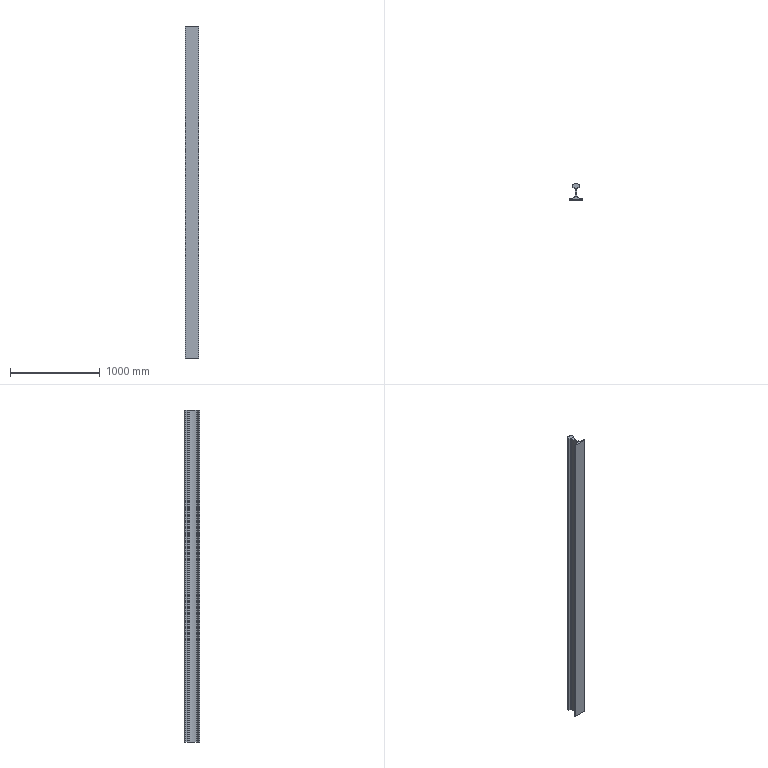Part | STEP file | 60 rail | 1 solid | 33 faces | box 150 x 176.167 x 3700 mm | volume 28206021 mm3 | cylinder 18 | plane 13 | spline 2 | commonest cylinder face diameters 4 x5 16 x2 26 x2 40 x2 50 x2 80 x2
STEP:
#1=CARTESIAN_POINT('',(-102.213,32.964,3700.));
#2=VERTEX_POINT('',#1);
#3=CARTESIAN_POINT('',(-103.574,34.86,3700.));
#4=VERTEX_POINT('',#3);
#5=CARTESIAN_POINT('',(-101.574,34.86,3700.));
#6=DIRECTION('',(0.,0.,-1.));
#7=DIRECTION('',(1.,0.,0.));
#8=AXIS2_PLACEMENT_3D('',#5,#6,#7);
#9=CIRCLE('',#8,2.);
#10=EDGE_CURVE('',#2,#4,#9,.T.);
#11=ORIENTED_EDGE('',*,*,#10,.T.);
#12=CARTESIAN_POINT('',(-103.574,34.86,0.));
#13=VERTEX_POINT('',#12);
#14=CARTESIAN_POINT('',(-103.574,34.86,3700.));
#15=DIRECTION('',(0.,0.,-1.));
#16=VECTOR('',#15,1000.);
#17=LINE('',#14,#16);
#18=EDGE_CURVE('',#4,#13,#17,.T.);
#19=ORIENTED_EDGE('',*,*,#18,.T.);
#20=CARTESIAN_POINT('',(-102.213,32.964,0.));
#21=VERTEX_POINT('',#20);
#22=CARTESIAN_POINT('',(-101.574,34.86,0.));
#23=DIRECTION('',(0.,0.,-1.));
#24=DIRECTION('',(1.,0.,0.));
#25=AXIS2_PLACEMENT_3D('',#22,#23,#24);
#26=CIRCLE('',#25,2.);
#27=EDGE_CURVE('',#21,#13,#26,.T.);
#28=ORIENTED_EDGE('',*,*,#27,.F.);
#29=CARTESIAN_POINT('',(-102.213,32.964,3700.));
#30=DIRECTION('',(0.,0.,-1.));
#31=VECTOR('',#30,1000.);
#32=LINE('',#29,#31);
#33=EDGE_CURVE('',#2,#21,#32,.T.);
#34=ORIENTED_EDGE('',*,*,#33,.F.);
#35=EDGE_LOOP('',(#11,#19,#28,#34));
#36=FACE_OUTER_BOUND('',#35,.T.);
#37=CARTESIAN_POINT('',(-101.574,34.86,3700.));
#38=DIRECTION('',(0.,0.,-1.));
#39=DIRECTION('',(-1.,0.,0.));
#40=AXIS2_PLACEMENT_3D('',#37,#38,#39);
#41=CYLINDRICAL_SURFACE('',#40,2.);
#42=ADVANCED_FACE('',(#36),#41,.T.);
#43=CARTESIAN_POINT('',(-80.306,23.184,0.));
#44=VERTEX_POINT('',#43);
#45=CARTESIAN_POINT('',(-77.547,14.047,0.));
#46=VERTEX_POINT('',#45);
#47=CARTESIAN_POINT('',(-102.419,11.522,0.));
#48=DIRECTION('',(0.,0.,-1.));
#49=DIRECTION('',(1.,0.,0.));
#50=AXIS2_PLACEMENT_3D('',#47,#48,#49);
#51=CIRCLE('',#50,25.);
#52=EDGE_CURVE('',#44,#46,#51,.T.);
#53=ORIENTED_EDGE('',*,*,#52,.T.);
#54=CARTESIAN_POINT('',(-77.547,14.047,3700.));
#55=VERTEX_POINT('',#54);
#56=CARTESIAN_POINT('',(-77.547,14.047,3700.));
#57=DIRECTION('',(0.,0.,-1.));
#58=VECTOR('',#57,1000.);
#59=LINE('',#56,#58);
#60=EDGE_CURVE('',#55,#46,#59,.T.);
#61=ORIENTED_EDGE('',*,*,#60,.F.);
#62=CARTESIAN_POINT('',(-80.306,23.184,3700.));
#63=VERTEX_POINT('',#62);
#64=CARTESIAN_POINT('',(-102.419,11.522,3700.));
#65=DIRECTION('',(0.,0.,-1.));
#66=DIRECTION('',(1.,0.,0.));
#67=AXIS2_PLACEMENT_3D('',#64,#65,#66);
#68=CIRCLE('',#67,25.);
#69=EDGE_CURVE('',#63,#55,#68,.T.);
#70=ORIENTED_EDGE('',*,*,#69,.F.);
#71=CARTESIAN_POINT('',(-80.306,23.184,3700.));
#72=DIRECTION('',(0.,0.,-1.));
#73=VECTOR('',#72,1000.);
#74=LINE('',#71,#73);
#75=EDGE_CURVE('',#63,#44,#74,.T.);
#76=ORIENTED_EDGE('',*,*,#75,.T.);
#77=EDGE_LOOP('',(#53,#61,#70,#76));
#78=FACE_OUTER_BOUND('',#77,.T.);
#79=CARTESIAN_POINT('',(-102.419,11.522,3700.));
#80=DIRECTION('',(0.,0.,-1.));
#81=DIRECTION('',(-1.,0.,0.));
#82=AXIS2_PLACEMENT_3D('',#79,#80,#81);
#83=CYLINDRICAL_SURFACE('',#82,25.);
#84=ADVANCED_FACE('',(#78),#83,.F.);
#85=CARTESIAN_POINT('',(-77.347,-66.653,0.));
#86=VERTEX_POINT('',#85);
#87=CARTESIAN_POINT('',(-77.547,14.047,0.));
#88=CARTESIAN_POINT('',(-70.798,-27.011,0.));
#89=CARTESIAN_POINT('',(-77.347,-66.653,0.));
#90=B_SPLINE_CURVE_WITH_KNOTS('',2,(#87,#88,#89),.UNSPECIFIED.,.F.,.F.,(3,3),(0.,0.7644),.UNSPECIFIED.);
#91=EDGE_CURVE('',#46,#86,#90,.T.);
#92=ORIENTED_EDGE('',*,*,#91,.T.);
#93=CARTESIAN_POINT('',(-77.347,-66.653,3700.));
#94=VERTEX_POINT('',#93);
#95=CARTESIAN_POINT('',(-77.347,-66.653,3700.));
#96=DIRECTION('',(0.,0.,-1.));
#97=VECTOR('',#96,1000.);
#98=LINE('',#95,#97);
#99=EDGE_CURVE('',#94,#86,#98,.T.);
#100=ORIENTED_EDGE('',*,*,#99,.F.);
#101=CARTESIAN_POINT('',(-77.547,14.047,3700.));
#102=CARTESIAN_POINT('',(-70.798,-27.011,3700.));
#103=CARTESIAN_POINT('',(-77.347,-66.653,3700.));
#104=B_SPLINE_CURVE_WITH_KNOTS('',2,(#101,#102,#103),.UNSPECIFIED.,.F.,.F.,(3,3),(0.,0.7644),.UNSPECIFIED.);
#105=EDGE_CURVE('',#55,#94,#104,.T.);
#106=ORIENTED_EDGE('',*,*,#105,.F.);
#107=ORIENTED_EDGE('',*,*,#60,.T.);
#108=EDGE_LOOP('',(#92,#100,#106,#107));
#109=FACE_OUTER_BOUND('',#108,.T.);
#110=CARTESIAN_POINT('',(-77.547,14.047,3700.));
#111=CARTESIAN_POINT('',(-77.547,14.047,0.));
#112=CARTESIAN_POINT('',(-70.798,-27.011,3700.));
#113=CARTESIAN_POINT('',(-70.798,-27.011,0.));
#114=CARTESIAN_POINT('',(-77.347,-66.653,3700.));
#115=CARTESIAN_POINT('',(-77.347,-66.653,0.));
#116=B_SPLINE_SURFACE_WITH_KNOTS('',2,1,((#110,#111),(#112,#113),(#114,#115)),.UNSPECIFIED.,.F.,.F.,.F.,(3,3),(2,2),(0.,0.7644),(0.,1.),.UNSPECIFIED.);
#117=ADVANCED_FACE('',(#109),#116,.F.);
#118=CARTESIAN_POINT('',(-90.947,-83.653,0.));
#119=VERTEX_POINT('',#118);
#120=CARTESIAN_POINT('',(-97.249,-64.671,0.));
#121=DIRECTION('',(0.,0.,-1.));
#122=DIRECTION('',(1.,0.,0.));
#123=AXIS2_PLACEMENT_3D('',#120,#121,#122);
#124=CIRCLE('',#123,20.);
#125=EDGE_CURVE('',#86,#119,#124,.T.);
#126=ORIENTED_EDGE('',*,*,#125,.T.);
#127=CARTESIAN_POINT('',(-90.947,-83.653,3700.));
#128=VERTEX_POINT('',#127);
#129=CARTESIAN_POINT('',(-90.947,-83.653,3700.));
#130=DIRECTION('',(0.,0.,-1.));
#131=VECTOR('',#130,1000.);
#132=LINE('',#129,#131);
#133=EDGE_CURVE('',#128,#119,#132,.T.);
#134=ORIENTED_EDGE('',*,*,#133,.F.);
#135=CARTESIAN_POINT('',(-97.249,-64.671,3700.));
#136=DIRECTION('',(0.,0.,-1.));
#137=DIRECTION('',(1.,0.,0.));
#138=AXIS2_PLACEMENT_3D('',#135,#136,#137);
#139=CIRCLE('',#138,20.);
#140=EDGE_CURVE('',#94,#128,#139,.T.);
#141=ORIENTED_EDGE('',*,*,#140,.F.);
#142=ORIENTED_EDGE('',*,*,#99,.T.);
#143=EDGE_LOOP('',(#126,#134,#141,#142));
#144=FACE_OUTER_BOUND('',#143,.T.);
#145=CARTESIAN_POINT('',(-97.249,-64.671,3700.));
#146=DIRECTION('',(0.,0.,-1.));
#147=DIRECTION('',(-1.,0.,0.));
#148=AXIS2_PLACEMENT_3D('',#145,#146,#147);
#149=CYLINDRICAL_SURFACE('',#148,20.);
#150=ADVANCED_FACE('',(#144),#149,.F.);
#151=CARTESIAN_POINT('',(-108.856,-89.622,0.));
#152=VERTEX_POINT('',#151);
#153=CARTESIAN_POINT('',(16.001,-48.003,0.));
#154=DIRECTION('',(-0.9487,-0.3162,0.));
#155=VECTOR('',#154,1000.);
#156=LINE('',#153,#155);
#157=EDGE_CURVE('',#119,#152,#156,.T.);
#158=ORIENTED_EDGE('',*,*,#157,.T.);
#159=CARTESIAN_POINT('',(-108.856,-89.622,3700.));
#160=VERTEX_POINT('',#159);
#161=CARTESIAN_POINT('',(-108.856,-89.622,3700.));
#162=DIRECTION('',(0.,0.,-1.));
#163=VECTOR('',#162,1000.);
#164=LINE('',#161,#163);
#165=EDGE_CURVE('',#160,#152,#164,.T.);
#166=ORIENTED_EDGE('',*,*,#165,.F.);
#167=CARTESIAN_POINT('',(16.001,-48.003,3700.));
#168=DIRECTION('',(-0.9487,-0.3162,0.));
#169=VECTOR('',#168,1000.);
#170=LINE('',#167,#169);
#171=EDGE_CURVE('',#128,#160,#170,.T.);
#172=ORIENTED_EDGE('',*,*,#171,.F.);
#173=ORIENTED_EDGE('',*,*,#133,.T.);
#174=EDGE_LOOP('',(#158,#166,#172,#173));
#175=FACE_OUTER_BOUND('',#174,.T.);
#176=CARTESIAN_POINT('',(16.001,-48.003,3700.));
#177=DIRECTION('',(0.3162,-0.9487,0.));
#178=DIRECTION('',(0.9487,0.3162,0.));
#179=AXIS2_PLACEMENT_3D('',#176,#177,#178);
#180=PLANE('',#179);
#181=ADVANCED_FACE('',(#175),#180,.F.);
#182=CARTESIAN_POINT('',(-117.028,-91.423,0.));
#183=VERTEX_POINT('',#182);
#184=CARTESIAN_POINT('',(-121.505,-51.675,0.));
#185=DIRECTION('',(0.,0.,1.));
#186=DIRECTION('',(1.,0.,0.));
#187=AXIS2_PLACEMENT_3D('',#184,#185,#186);
#188=CIRCLE('',#187,40.);
#189=EDGE_CURVE('',#183,#152,#188,.T.);
#190=ORIENTED_EDGE('',*,*,#189,.F.);
#191=CARTESIAN_POINT('',(-117.028,-91.423,3700.));
#192=VERTEX_POINT('',#191);
#193=CARTESIAN_POINT('',(-117.028,-91.423,3700.));
#194=DIRECTION('',(0.,0.,-1.));
#195=VECTOR('',#194,1000.);
#196=LINE('',#193,#195);
#197=EDGE_CURVE('',#192,#183,#196,.T.);
#198=ORIENTED_EDGE('',*,*,#197,.F.);
#199=CARTESIAN_POINT('',(-121.505,-51.675,3700.));
#200=DIRECTION('',(0.,0.,1.));
#201=DIRECTION('',(1.,0.,0.));
#202=AXIS2_PLACEMENT_3D('',#199,#200,#201);
#203=CIRCLE('',#202,40.);
#204=EDGE_CURVE('',#192,#160,#203,.T.);
#205=ORIENTED_EDGE('',*,*,#204,.T.);
#206=ORIENTED_EDGE('',*,*,#165,.T.);
#207=EDGE_LOOP('',(#190,#198,#205,#206));
#208=FACE_OUTER_BOUND('',#207,.T.);
#209=CARTESIAN_POINT('',(-121.505,-51.675,3700.));
#210=DIRECTION('',(0.,0.,-1.));
#211=DIRECTION('',(-1.,0.,0.));
#212=AXIS2_PLACEMENT_3D('',#209,#210,#211);
#213=CYLINDRICAL_SURFACE('',#212,40.);
#214=ADVANCED_FACE('',(#208),#213,.F.);
#215=CARTESIAN_POINT('',(-140.371,-94.052,0.));
#216=VERTEX_POINT('',#215);
#217=CARTESIAN_POINT('',(8.702,-77.263,0.));
#218=DIRECTION('',(-0.9937,-0.1119,0.));
#219=VECTOR('',#218,1000.);
#220=LINE('',#217,#219);
#221=EDGE_CURVE('',#183,#216,#220,.T.);
#222=ORIENTED_EDGE('',*,*,#221,.T.);
#223=CARTESIAN_POINT('',(-140.371,-94.052,3700.));
#224=VERTEX_POINT('',#223);
#225=CARTESIAN_POINT('',(-140.371,-94.052,3700.));
#226=DIRECTION('',(0.,0.,-1.));
#227=VECTOR('',#226,1000.);
#228=LINE('',#225,#227);
#229=EDGE_CURVE('',#224,#216,#228,.T.);
#230=ORIENTED_EDGE('',*,*,#229,.F.);
#231=CARTESIAN_POINT('',(8.702,-77.263,3700.));
#232=DIRECTION('',(-0.9937,-0.1119,0.));
#233=VECTOR('',#232,1000.);
#234=LINE('',#231,#233);
#235=EDGE_CURVE('',#192,#224,#234,.T.);
#236=ORIENTED_EDGE('',*,*,#235,.F.);
#237=ORIENTED_EDGE('',*,*,#197,.T.);
#238=EDGE_LOOP('',(#222,#230,#236,#237));
#239=FACE_OUTER_BOUND('',#238,.T.);
#240=CARTESIAN_POINT('',(8.702,-77.263,3700.));
#241=DIRECTION('',(0.1119,-0.9937,0.));
#242=DIRECTION('',(0.9937,0.1119,0.));
#243=AXIS2_PLACEMENT_3D('',#240,#241,#242);
#244=PLANE('',#243);
#245=ADVANCED_FACE('',(#239),#244,.F.);
#246=CARTESIAN_POINT('',(-142.147,-96.04,0.));
#247=VERTEX_POINT('',#246);
#248=CARTESIAN_POINT('',(-140.147,-96.04,0.));
#249=DIRECTION('',(0.,0.,-1.));
#250=DIRECTION('',(1.,0.,0.));
#251=AXIS2_PLACEMENT_3D('',#248,#249,#250);
#252=CIRCLE('',#251,2.);
#253=EDGE_CURVE('',#247,#216,#252,.T.);
#254=ORIENTED_EDGE('',*,*,#253,.F.);
#255=CARTESIAN_POINT('',(-142.147,-96.04,3700.));
#256=VERTEX_POINT('',#255);
#257=CARTESIAN_POINT('',(-142.147,-96.04,3700.));
#258=DIRECTION('',(0.,0.,-1.));
#259=VECTOR('',#258,1000.);
#260=LINE('',#257,#259);
#261=EDGE_CURVE('',#256,#247,#260,.T.);
#262=ORIENTED_EDGE('',*,*,#261,.F.);
#263=CARTESIAN_POINT('',(-140.147,-96.04,3700.));
#264=DIRECTION('',(0.,0.,-1.));
#265=DIRECTION('',(1.,0.,0.));
#266=AXIS2_PLACEMENT_3D('',#263,#264,#265);
#267=CIRCLE('',#266,2.);
#268=EDGE_CURVE('',#256,#224,#267,.T.);
#269=ORIENTED_EDGE('',*,*,#268,.T.);
#270=ORIENTED_EDGE('',*,*,#229,.T.);
#271=EDGE_LOOP('',(#254,#262,#269,#270));
#272=FACE_OUTER_BOUND('',#271,.T.);
#273=CARTESIAN_POINT('',(-140.147,-96.04,3700.));
#274=DIRECTION('',(0.,0.,-1.));
#275=DIRECTION('',(-1.,0.,0.));
#276=AXIS2_PLACEMENT_3D('',#273,#274,#275);
#277=CYLINDRICAL_SURFACE('',#276,2.);
#278=ADVANCED_FACE('',(#272),#277,.T.);
#279=CARTESIAN_POINT('',(-142.147,-106.253,0.));
#280=VERTEX_POINT('',#279);
#281=CARTESIAN_POINT('',(-142.147,0.,0.));
#282=DIRECTION('',(0.,1.,0.));
#283=VECTOR('',#282,1000.);
#284=LINE('',#281,#283);
#285=EDGE_CURVE('',#280,#247,#284,.T.);
#286=ORIENTED_EDGE('',*,*,#285,.F.);
#287=CARTESIAN_POINT('',(-142.147,-106.253,3700.));
#288=VERTEX_POINT('',#287);
#289=CARTESIAN_POINT('',(-142.147,-106.253,3700.));
#290=DIRECTION('',(0.,0.,-1.));
#291=VECTOR('',#290,1000.);
#292=LINE('',#289,#291);
#293=EDGE_CURVE('',#288,#280,#292,.T.);
#294=ORIENTED_EDGE('',*,*,#293,.F.);
#295=CARTESIAN_POINT('',(-142.147,0.,3700.));
#296=DIRECTION('',(0.,1.,0.));
#297=VECTOR('',#296,1000.);
#298=LINE('',#295,#297);
#299=EDGE_CURVE('',#288,#256,#298,.T.);
#300=ORIENTED_EDGE('',*,*,#299,.T.);
#301=ORIENTED_EDGE('',*,*,#261,.T.);
#302=EDGE_LOOP('',(#286,#294,#300,#301));
#303=FACE_OUTER_BOUND('',#302,.T.);
#304=CARTESIAN_POINT('',(-142.147,0.,3700.));
#305=DIRECTION('',(-1.,0.,0.));
#306=DIRECTION('',(0.,0.,1.));
#307=AXIS2_PLACEMENT_3D('',#304,#305,#306);
#308=PLANE('',#307);
#309=ADVANCED_FACE('',(#303),#308,.T.);
#310=CARTESIAN_POINT('',(7.853,-106.253,0.));
#311=VERTEX_POINT('',#310);
#312=CARTESIAN_POINT('',(0.,-106.253,0.));
#313=DIRECTION('',(1.,0.,0.));
#314=VECTOR('',#313,1000.);
#315=LINE('',#312,#314);
#316=EDGE_CURVE('',#280,#311,#315,.T.);
#317=ORIENTED_EDGE('',*,*,#316,.T.);
#318=CARTESIAN_POINT('',(7.853,-106.253,3700.));
#319=VERTEX_POINT('',#318);
#320=CARTESIAN_POINT('',(7.853,-106.253,3700.));
#321=DIRECTION('',(0.,0.,-1.));
#322=VECTOR('',#321,1000.);
#323=LINE('',#320,#322);
#324=EDGE_CURVE('',#319,#311,#323,.T.);
#325=ORIENTED_EDGE('',*,*,#324,.F.);
#326=CARTESIAN_POINT('',(0.,-106.253,3700.));
#327=DIRECTION('',(1.,0.,0.));
#328=VECTOR('',#327,1000.);
#329=LINE('',#326,#328);
#330=EDGE_CURVE('',#288,#319,#329,.T.);
#331=ORIENTED_EDGE('',*,*,#330,.F.);
#332=ORIENTED_EDGE('',*,*,#293,.T.);
#333=EDGE_LOOP('',(#317,#325,#331,#332));
#334=FACE_OUTER_BOUND('',#333,.T.);
#335=CARTESIAN_POINT('',(0.,-106.253,3700.));
#336=DIRECTION('',(0.,1.,0.));
#337=DIRECTION('',(0.,0.,1.));
#338=AXIS2_PLACEMENT_3D('',#335,#336,#337);
#339=PLANE('',#338);
#340=ADVANCED_FACE('',(#334),#339,.F.);
#341=CARTESIAN_POINT('',(7.853,-96.04,0.));
#342=VERTEX_POINT('',#341);
#343=CARTESIAN_POINT('',(7.853,0.,0.));
#344=DIRECTION('',(0.,1.,0.));
#345=VECTOR('',#344,1000.);
#346=LINE('',#343,#345);
#347=EDGE_CURVE('',#311,#342,#346,.T.);
#348=ORIENTED_EDGE('',*,*,#347,.T.);
#349=CARTESIAN_POINT('',(7.853,-96.04,3700.));
#350=VERTEX_POINT('',#349);
#351=CARTESIAN_POINT('',(7.853,-96.04,3700.));
#352=DIRECTION('',(0.,0.,-1.));
#353=VECTOR('',#352,1000.);
#354=LINE('',#351,#353);
#355=EDGE_CURVE('',#350,#342,#354,.T.);
#356=ORIENTED_EDGE('',*,*,#355,.F.);
#357=CARTESIAN_POINT('',(7.853,0.,3700.));
#358=DIRECTION('',(0.,1.,0.));
#359=VECTOR('',#358,1000.);
#360=LINE('',#357,#359);
#361=EDGE_CURVE('',#319,#350,#360,.T.);
#362=ORIENTED_EDGE('',*,*,#361,.F.);
#363=ORIENTED_EDGE('',*,*,#324,.T.);
#364=EDGE_LOOP('',(#348,#356,#362,#363));
#365=FACE_OUTER_BOUND('',#364,.T.);
#366=CARTESIAN_POINT('',(7.853,0.,3700.));
#367=DIRECTION('',(-1.,0.,0.));
#368=DIRECTION('',(0.,0.,1.));
#369=AXIS2_PLACEMENT_3D('',#366,#367,#368);
#370=PLANE('',#369);
#371=ADVANCED_FACE('',(#365),#370,.F.);
#372=CARTESIAN_POINT('',(6.077,-94.052,0.));
#373=VERTEX_POINT('',#372);
#374=CARTESIAN_POINT('',(5.853,-96.04,0.));
#375=DIRECTION('',(0.,0.,1.));
#376=DIRECTION('',(1.,0.,0.));
#377=AXIS2_PLACEMENT_3D('',#374,#375,#376);
#378=CIRCLE('',#377,2.);
#379=EDGE_CURVE('',#342,#373,#378,.T.);
#380=ORIENTED_EDGE('',*,*,#379,.T.);
#381=CARTESIAN_POINT('',(6.077,-94.052,3700.));
#382=VERTEX_POINT('',#381);
#383=CARTESIAN_POINT('',(6.077,-94.052,3700.));
#384=DIRECTION('',(0.,0.,-1.));
#385=VECTOR('',#384,1000.);
#386=LINE('',#383,#385);
#387=EDGE_CURVE('',#382,#373,#386,.T.);
#388=ORIENTED_EDGE('',*,*,#387,.F.);
#389=CARTESIAN_POINT('',(5.853,-96.04,3700.));
#390=DIRECTION('',(0.,0.,1.));
#391=DIRECTION('',(1.,0.,0.));
#392=AXIS2_PLACEMENT_3D('',#389,#390,#391);
#393=CIRCLE('',#392,2.);
#394=EDGE_CURVE('',#350,#382,#393,.T.);
#395=ORIENTED_EDGE('',*,*,#394,.F.);
#396=ORIENTED_EDGE('',*,*,#355,.T.);
#397=EDGE_LOOP('',(#380,#388,#395,#396));
#398=FACE_OUTER_BOUND('',#397,.T.);
#399=CARTESIAN_POINT('',(5.853,-96.04,3700.));
#400=DIRECTION('',(0.,0.,-1.));
#401=DIRECTION('',(-1.,0.,0.));
#402=AXIS2_PLACEMENT_3D('',#399,#400,#401);
#403=CYLINDRICAL_SURFACE('',#402,2.);
#404=ADVANCED_FACE('',(#398),#403,.T.);
#405=CARTESIAN_POINT('',(-17.266,-91.423,0.));
#406=VERTEX_POINT('',#405);
#407=CARTESIAN_POINT('',(-10.384,-92.199,0.));
#408=DIRECTION('',(0.9937,-0.1119,0.));
#409=VECTOR('',#408,1000.);
#410=LINE('',#407,#409);
#411=EDGE_CURVE('',#406,#373,#410,.T.);
#412=ORIENTED_EDGE('',*,*,#411,.F.);
#413=CARTESIAN_POINT('',(-17.266,-91.423,3700.));
#414=VERTEX_POINT('',#413);
#415=CARTESIAN_POINT('',(-17.266,-91.423,3700.));
#416=DIRECTION('',(0.,0.,-1.));
#417=VECTOR('',#416,1000.);
#418=LINE('',#415,#417);
#419=EDGE_CURVE('',#414,#406,#418,.T.);
#420=ORIENTED_EDGE('',*,*,#419,.F.);
#421=CARTESIAN_POINT('',(-10.384,-92.199,3700.));
#422=DIRECTION('',(0.9937,-0.1119,0.));
#423=VECTOR('',#422,1000.);
#424=LINE('',#421,#423);
#425=EDGE_CURVE('',#414,#382,#424,.T.);
#426=ORIENTED_EDGE('',*,*,#425,.T.);
#427=ORIENTED_EDGE('',*,*,#387,.T.);
#428=EDGE_LOOP('',(#412,#420,#426,#427));
#429=FACE_OUTER_BOUND('',#428,.T.);
#430=CARTESIAN_POINT('',(-10.384,-92.199,3700.));
#431=DIRECTION('',(0.1119,0.9937,0.));
#432=DIRECTION('',(-0.9937,0.1119,0.));
#433=AXIS2_PLACEMENT_3D('',#430,#431,#432);
#434=PLANE('',#433);
#435=ADVANCED_FACE('',(#429),#434,.T.);
#436=CARTESIAN_POINT('',(-25.438,-89.622,0.));
#437=VERTEX_POINT('',#436);
#438=CARTESIAN_POINT('',(-12.789,-51.675,0.));
#439=DIRECTION('',(0.,0.,-1.));
#440=DIRECTION('',(1.,0.,0.));
#441=AXIS2_PLACEMENT_3D('',#438,#439,#440);
#442=CIRCLE('',#441,40.);
#443=EDGE_CURVE('',#406,#437,#442,.T.);
#444=ORIENTED_EDGE('',*,*,#443,.T.);
#445=CARTESIAN_POINT('',(-25.438,-89.622,3700.));
#446=VERTEX_POINT('',#445);
#447=CARTESIAN_POINT('',(-25.438,-89.622,3700.));
#448=DIRECTION('',(0.,0.,-1.));
#449=VECTOR('',#448,1000.);
#450=LINE('',#447,#449);
#451=EDGE_CURVE('',#446,#437,#450,.T.);
#452=ORIENTED_EDGE('',*,*,#451,.F.);
#453=CARTESIAN_POINT('',(-12.789,-51.675,3700.));
#454=DIRECTION('',(0.,0.,-1.));
#455=DIRECTION('',(1.,0.,0.));
#456=AXIS2_PLACEMENT_3D('',#453,#454,#455);
#457=CIRCLE('',#456,40.);
#458=EDGE_CURVE('',#414,#446,#457,.T.);
#459=ORIENTED_EDGE('',*,*,#458,.F.);
#460=ORIENTED_EDGE('',*,*,#419,.T.);
#461=EDGE_LOOP('',(#444,#452,#459,#460));
#462=FACE_OUTER_BOUND('',#461,.T.);
#463=CARTESIAN_POINT('',(-12.789,-51.675,3700.));
#464=DIRECTION('',(0.,0.,-1.));
#465=DIRECTION('',(-1.,0.,0.));
#466=AXIS2_PLACEMENT_3D('',#463,#464,#465);
#467=CYLINDRICAL_SURFACE('',#466,40.);
#468=ADVANCED_FACE('',(#462),#467,.F.);
#469=CARTESIAN_POINT('',(-43.347,-83.653,0.));
#470=VERTEX_POINT('',#469);
#471=CARTESIAN_POINT('',(-29.43,-88.291,0.));
#472=DIRECTION('',(0.9487,-0.3162,0.));
#473=VECTOR('',#472,1000.);
#474=LINE('',#471,#473);
#475=EDGE_CURVE('',#470,#437,#474,.T.);
#476=ORIENTED_EDGE('',*,*,#475,.F.);
#477=CARTESIAN_POINT('',(-43.347,-83.653,3700.));
#478=VERTEX_POINT('',#477);
#479=CARTESIAN_POINT('',(-43.347,-83.653,3700.));
#480=DIRECTION('',(0.,0.,-1.));
#481=VECTOR('',#480,1000.);
#482=LINE('',#479,#481);
#483=EDGE_CURVE('',#478,#470,#482,.T.);
#484=ORIENTED_EDGE('',*,*,#483,.F.);
#485=CARTESIAN_POINT('',(-29.43,-88.291,3700.));
#486=DIRECTION('',(0.9487,-0.3162,0.));
#487=VECTOR('',#486,1000.);
#488=LINE('',#485,#487);
#489=EDGE_CURVE('',#478,#446,#488,.T.);
#490=ORIENTED_EDGE('',*,*,#489,.T.);
#491=ORIENTED_EDGE('',*,*,#451,.T.);
#492=EDGE_LOOP('',(#476,#484,#490,#491));
#493=FACE_OUTER_BOUND('',#492,.T.);
#494=CARTESIAN_POINT('',(-29.43,-88.291,3700.));
#495=DIRECTION('',(0.3162,0.9487,0.));
#496=DIRECTION('',(-0.9487,0.3162,0.));
#497=AXIS2_PLACEMENT_3D('',#494,#495,#496);
#498=PLANE('',#497);
#499=ADVANCED_FACE('',(#493),#498,.T.);
#500=CARTESIAN_POINT('',(-56.947,-66.653,0.));
#501=VERTEX_POINT('',#500);
#502=CARTESIAN_POINT('',(-37.045,-64.671,0.));
#503=DIRECTION('',(0.,0.,1.));
#504=DIRECTION('',(1.,0.,0.));
#505=AXIS2_PLACEMENT_3D('',#502,#503,#504);
#506=CIRCLE('',#505,20.);
#507=EDGE_CURVE('',#501,#470,#506,.T.);
#508=ORIENTED_EDGE('',*,*,#507,.F.);
#509=CARTESIAN_POINT('',(-56.947,-66.653,3700.));
#510=VERTEX_POINT('',#509);
#511=CARTESIAN_POINT('',(-56.947,-66.653,3700.));
#512=DIRECTION('',(0.,0.,-1.));
#513=VECTOR('',#512,1000.);
#514=LINE('',#511,#513);
#515=EDGE_CURVE('',#510,#501,#514,.T.);
#516=ORIENTED_EDGE('',*,*,#515,.F.);
#517=CARTESIAN_POINT('',(-37.045,-64.671,3700.));
#518=DIRECTION('',(0.,0.,1.));
#519=DIRECTION('',(1.,0.,0.));
#520=AXIS2_PLACEMENT_3D('',#517,#518,#519);
#521=CIRCLE('',#520,20.);
#522=EDGE_CURVE('',#510,#478,#521,.T.);
#523=ORIENTED_EDGE('',*,*,#522,.T.);
#524=ORIENTED_EDGE('',*,*,#483,.T.);
#525=EDGE_LOOP('',(#508,#516,#523,#524));
#526=FACE_OUTER_BOUND('',#525,.T.);
#527=CARTESIAN_POINT('',(-37.045,-64.671,3700.));
#528=DIRECTION('',(0.,0.,-1.));
#529=DIRECTION('',(-1.,0.,0.));
#530=AXIS2_PLACEMENT_3D('',#527,#528,#529);
#531=CYLINDRICAL_SURFACE('',#530,20.);
#532=ADVANCED_FACE('',(#526),#531,.F.);
#533=CARTESIAN_POINT('',(-56.747,14.047,0.));
#534=VERTEX_POINT('',#533);
#535=CARTESIAN_POINT('',(-56.747,14.047,0.));
#536=CARTESIAN_POINT('',(-63.496,-27.011,0.));
#537=CARTESIAN_POINT('',(-56.947,-66.653,0.));
#538=B_SPLINE_CURVE_WITH_KNOTS('',2,(#535,#536,#537),.UNSPECIFIED.,.F.,.F.,(3,3),(0.,0.7644),.UNSPECIFIED.);
#539=EDGE_CURVE('',#534,#501,#538,.T.);
#540=ORIENTED_EDGE('',*,*,#539,.F.);
#541=CARTESIAN_POINT('',(-56.747,14.047,3700.));
#542=VERTEX_POINT('',#541);
#543=CARTESIAN_POINT('',(-56.747,14.047,3700.));
#544=DIRECTION('',(0.,0.,-1.));
#545=VECTOR('',#544,1000.);
#546=LINE('',#543,#545);
#547=EDGE_CURVE('',#542,#534,#546,.T.);
#548=ORIENTED_EDGE('',*,*,#547,.F.);
#549=CARTESIAN_POINT('',(-56.747,14.047,3700.));
#550=CARTESIAN_POINT('',(-63.496,-27.011,3700.));
#551=CARTESIAN_POINT('',(-56.947,-66.653,3700.));
#552=B_SPLINE_CURVE_WITH_KNOTS('',2,(#549,#550,#551),.UNSPECIFIED.,.F.,.F.,(3,3),(0.,0.7644),.UNSPECIFIED.);
#553=EDGE_CURVE('',#542,#510,#552,.T.);
#554=ORIENTED_EDGE('',*,*,#553,.T.);
#555=ORIENTED_EDGE('',*,*,#515,.T.);
#556=EDGE_LOOP('',(#540,#548,#554,#555));
#557=FACE_OUTER_BOUND('',#556,.T.);
#558=CARTESIAN_POINT('',(-56.747,14.047,3700.));
#559=CARTESIAN_POINT('',(-56.747,14.047,0.));
#560=CARTESIAN_POINT('',(-63.496,-27.011,3700.));
#561=CARTESIAN_POINT('',(-63.496,-27.011,0.));
#562=CARTESIAN_POINT('',(-56.947,-66.653,3700.));
#563=CARTESIAN_POINT('',(-56.947,-66.653,0.));
#564=B_SPLINE_SURFACE_WITH_KNOTS('',2,1,((#558,#559),(#560,#561),(#562,#563)),.UNSPECIFIED.,.F.,.F.,.F.,(3,3),(2,2),(0.,0.7644),(0.,1.),.UNSPECIFIED.);
#565=ADVANCED_FACE('',(#557),#564,.T.);
#566=CARTESIAN_POINT('',(-53.988,23.184,0.));
#567=VERTEX_POINT('',#566);
#568=CARTESIAN_POINT('',(-31.875,11.522,0.));
#569=DIRECTION('',(0.,0.,1.));
#570=DIRECTION('',(1.,0.,0.));
#571=AXIS2_PLACEMENT_3D('',#568,#569,#570);
#572=CIRCLE('',#571,25.);
#573=EDGE_CURVE('',#567,#534,#572,.T.);
#574=ORIENTED_EDGE('',*,*,#573,.F.);
#575=CARTESIAN_POINT('',(-53.988,23.184,3700.));
#576=VERTEX_POINT('',#575);
#577=CARTESIAN_POINT('',(-53.988,23.184,3700.));
#578=DIRECTION('',(0.,0.,-1.));
#579=VECTOR('',#578,1000.);
#580=LINE('',#577,#579);
#581=EDGE_CURVE('',#576,#567,#580,.T.);
#582=ORIENTED_EDGE('',*,*,#581,.F.);
#583=CARTESIAN_POINT('',(-31.875,11.522,3700.));
#584=DIRECTION('',(0.,0.,1.));
#585=DIRECTION('',(1.,0.,0.));
#586=AXIS2_PLACEMENT_3D('',#583,#584,#585);
#587=CIRCLE('',#586,25.);
#588=EDGE_CURVE('',#576,#542,#587,.T.);
#589=ORIENTED_EDGE('',*,*,#588,.T.);
#590=ORIENTED_EDGE('',*,*,#547,.T.);
#591=EDGE_LOOP('',(#574,#582,#589,#590));
#592=FACE_OUTER_BOUND('',#591,.T.);
#593=CARTESIAN_POINT('',(-31.875,11.522,3700.));
#594=DIRECTION('',(0.,0.,-1.));
#595=DIRECTION('',(-1.,0.,0.));
#596=AXIS2_PLACEMENT_3D('',#593,#594,#595);
#597=CYLINDRICAL_SURFACE('',#596,25.);
#598=ADVANCED_FACE('',(#592),#597,.F.);
#599=CARTESIAN_POINT('',(-49.347,27.147,0.));
#600=VERTEX_POINT('',#599);
#601=CARTESIAN_POINT('',(-46.865,19.542,0.));
#602=DIRECTION('',(0.,0.,1.));
#603=DIRECTION('',(1.,0.,0.));
#604=AXIS2_PLACEMENT_3D('',#601,#602,#603);
#605=CIRCLE('',#604,8.);
#606=EDGE_CURVE('',#600,#567,#605,.T.);
#607=ORIENTED_EDGE('',*,*,#606,.F.);
#608=CARTESIAN_POINT('',(-49.347,27.147,3700.));
#609=VERTEX_POINT('',#608);
#610=CARTESIAN_POINT('',(-49.347,27.147,3700.));
#611=DIRECTION('',(0.,0.,-1.));
#612=VECTOR('',#611,1000.);
#613=LINE('',#610,#612);
#614=EDGE_CURVE('',#609,#600,#613,.T.);
#615=ORIENTED_EDGE('',*,*,#614,.F.);
#616=CARTESIAN_POINT('',(-46.865,19.542,3700.));
#617=DIRECTION('',(0.,0.,1.));
#618=DIRECTION('',(1.,0.,0.));
#619=AXIS2_PLACEMENT_3D('',#616,#617,#618);
#620=CIRCLE('',#619,8.);
#621=EDGE_CURVE('',#609,#576,#620,.T.);
#622=ORIENTED_EDGE('',*,*,#621,.T.);
#623=ORIENTED_EDGE('',*,*,#581,.T.);
#624=EDGE_LOOP('',(#607,#615,#622,#623));
#625=FACE_OUTER_BOUND('',#624,.T.);
#626=CARTESIAN_POINT('',(-46.865,19.542,3700.));
#627=DIRECTION('',(0.,0.,-1.));
#628=DIRECTION('',(-1.,0.,0.));
#629=AXIS2_PLACEMENT_3D('',#626,#627,#628);
#630=CYLINDRICAL_SURFACE('',#629,8.);
#631=ADVANCED_FACE('',(#625),#630,.F.);
#632=CARTESIAN_POINT('',(-32.081,32.964,0.));
#633=VERTEX_POINT('',#632);
#634=CARTESIAN_POINT('',(-13.244,39.311,0.));
#635=DIRECTION('',(0.9477,0.3193,0.));
#636=VECTOR('',#635,1000.);
#637=LINE('',#634,#636);
#638=EDGE_CURVE('',#600,#633,#637,.T.);
#639=ORIENTED_EDGE('',*,*,#638,.T.);
#640=CARTESIAN_POINT('',(-32.081,32.964,3700.));
#641=VERTEX_POINT('',#640);
#642=CARTESIAN_POINT('',(-32.081,32.964,3700.));
#643=DIRECTION('',(0.,0.,-1.));
#644=VECTOR('',#643,1000.);
#645=LINE('',#642,#644);
#646=EDGE_CURVE('',#641,#633,#645,.T.);
#647=ORIENTED_EDGE('',*,*,#646,.F.);
#648=CARTESIAN_POINT('',(-13.244,39.311,3700.));
#649=DIRECTION('',(0.9477,0.3193,0.));
#650=VECTOR('',#649,1000.);
#651=LINE('',#648,#650);
#652=EDGE_CURVE('',#609,#641,#651,.T.);
#653=ORIENTED_EDGE('',*,*,#652,.F.);
#654=ORIENTED_EDGE('',*,*,#614,.T.);
#655=EDGE_LOOP('',(#639,#647,#653,#654));
#656=FACE_OUTER_BOUND('',#655,.T.);
#657=CARTESIAN_POINT('',(-13.244,39.311,3700.));
#658=DIRECTION('',(-0.3193,0.9477,0.));
#659=DIRECTION('',(-0.9477,-0.3193,0.));
#660=AXIS2_PLACEMENT_3D('',#657,#658,#659);
#661=PLANE('',#660);
#662=ADVANCED_FACE('',(#656),#661,.F.);
#663=CARTESIAN_POINT('',(-30.722,34.959,0.));
#664=VERTEX_POINT('',#663);
#665=CARTESIAN_POINT('',(-32.72,34.86,0.));
#666=DIRECTION('',(0.,0.,1.));
#667=DIRECTION('',(1.,0.,0.));
#668=AXIS2_PLACEMENT_3D('',#665,#666,#667);
#669=CIRCLE('',#668,2.);
#670=EDGE_CURVE('',#633,#664,#669,.T.);
#671=ORIENTED_EDGE('',*,*,#670,.T.);
#672=CARTESIAN_POINT('',(-30.722,34.959,3700.));
#673=VERTEX_POINT('',#672);
#674=CARTESIAN_POINT('',(-30.722,34.959,3700.));
#675=DIRECTION('',(0.,0.,-1.));
#676=VECTOR('',#675,1000.);
#677=LINE('',#674,#676);
#678=EDGE_CURVE('',#673,#664,#677,.T.);
#679=ORIENTED_EDGE('',*,*,#678,.F.);
#680=CARTESIAN_POINT('',(-32.72,34.86,3700.));
#681=DIRECTION('',(0.,0.,1.));
#682=DIRECTION('',(1.,0.,0.));
#683=AXIS2_PLACEMENT_3D('',#680,#681,#682);
#684=CIRCLE('',#683,2.);
#685=EDGE_CURVE('',#641,#673,#684,.T.);
#686=ORIENTED_EDGE('',*,*,#685,.F.);
#687=ORIENTED_EDGE('',*,*,#646,.T.);
#688=EDGE_LOOP('',(#671,#679,#686,#687));
#689=FACE_OUTER_BOUND('',#688,.T.);
#690=CARTESIAN_POINT('',(-32.72,34.86,3700.));
#691=DIRECTION('',(0.,0.,-1.));
#692=DIRECTION('',(-1.,0.,0.));
#693=AXIS2_PLACEMENT_3D('',#690,#691,#692);
#694=CYLINDRICAL_SURFACE('',#693,2.);
#695=ADVANCED_FACE('',(#689),#694,.T.);
#696=CARTESIAN_POINT('',(-31.747,55.547,0.));
#697=VERTEX_POINT('',#696);
#698=CARTESIAN_POINT('',(-28.911,-1.439,0.));
#699=DIRECTION('',(0.04971,-0.9988,0.));
#700=VECTOR('',#699,1000.);
#701=LINE('',#698,#700);
#702=EDGE_CURVE('',#697,#664,#701,.T.);
#703=ORIENTED_EDGE('',*,*,#702,.F.);
#704=CARTESIAN_POINT('',(-31.747,55.547,3700.));
#705=VERTEX_POINT('',#704);
#706=CARTESIAN_POINT('',(-31.747,55.547,3700.));
#707=DIRECTION('',(0.,0.,-1.));
#708=VECTOR('',#707,1000.);
#709=LINE('',#706,#708);
#710=EDGE_CURVE('',#705,#697,#709,.T.);
#711=ORIENTED_EDGE('',*,*,#710,.F.);
#712=CARTESIAN_POINT('',(-28.911,-1.439,3700.));
#713=DIRECTION('',(0.04971,-0.9988,0.));
#714=VECTOR('',#713,1000.);
#715=LINE('',#712,#714);
#716=EDGE_CURVE('',#705,#673,#715,.T.);
#717=ORIENTED_EDGE('',*,*,#716,.T.);
#718=ORIENTED_EDGE('',*,*,#678,.T.);
#719=EDGE_LOOP('',(#703,#711,#717,#718));
#720=FACE_OUTER_BOUND('',#719,.T.);
#721=CARTESIAN_POINT('',(-28.911,-1.439,3700.));
#722=DIRECTION('',(0.9988,0.04971,0.));
#723=DIRECTION('',(-0.04971,0.9988,0.));
#724=AXIS2_PLACEMENT_3D('',#721,#722,#723);
#725=PLANE('',#724);
#726=ADVANCED_FACE('',(#720),#725,.T.);
#727=CARTESIAN_POINT('',(-41.44,67.459,0.));
#728=VERTEX_POINT('',#727);
#729=CARTESIAN_POINT('',(-44.73,54.883,0.));
#730=DIRECTION('',(0.,0.,1.));
#731=DIRECTION('',(1.,0.,0.));
#732=AXIS2_PLACEMENT_3D('',#729,#730,#731);
#733=CIRCLE('',#732,13.);
#734=EDGE_CURVE('',#697,#728,#733,.T.);
#735=ORIENTED_EDGE('',*,*,#734,.T.);
#736=CARTESIAN_POINT('',(-41.44,67.459,3700.));
#737=VERTEX_POINT('',#736);
#738=CARTESIAN_POINT('',(-41.44,67.459,3700.));
#739=DIRECTION('',(0.,0.,-1.));
#740=VECTOR('',#739,1000.);
#741=LINE('',#738,#740);
#742=EDGE_CURVE('',#737,#728,#741,.T.);
#743=ORIENTED_EDGE('',*,*,#742,.F.);
#744=CARTESIAN_POINT('',(-44.73,54.883,3700.));
#745=DIRECTION('',(0.,0.,1.));
#746=DIRECTION('',(1.,0.,0.));
#747=AXIS2_PLACEMENT_3D('',#744,#745,#746);
#748=CIRCLE('',#747,13.);
#749=EDGE_CURVE('',#705,#737,#748,.T.);
#750=ORIENTED_EDGE('',*,*,#749,.F.);
#751=ORIENTED_EDGE('',*,*,#710,.T.);
#752=EDGE_LOOP('',(#735,#743,#750,#751));
#753=FACE_OUTER_BOUND('',#752,.T.);
#754=CARTESIAN_POINT('',(-44.73,54.883,3700.));
#755=DIRECTION('',(0.,0.,-1.));
#756=DIRECTION('',(-1.,0.,0.));
#757=AXIS2_PLACEMENT_3D('',#754,#755,#756);
#758=CYLINDRICAL_SURFACE('',#757,13.);
#759=ADVANCED_FACE('',(#753),#758,.T.);
#760=CARTESIAN_POINT('',(-57.147,69.747,0.));
#761=VERTEX_POINT('',#760);
#762=CARTESIAN_POINT('',(-60.768,-10.171,0.));
#763=DIRECTION('',(0.,0.,1.));
#764=DIRECTION('',(1.,0.,0.));
#765=AXIS2_PLACEMENT_3D('',#762,#763,#764);
#766=CIRCLE('',#765,80.);
#767=EDGE_CURVE('',#728,#761,#766,.T.);
#768=ORIENTED_EDGE('',*,*,#767,.T.);
#769=CARTESIAN_POINT('',(-57.147,69.747,3700.));
#770=VERTEX_POINT('',#769);
#771=CARTESIAN_POINT('',(-57.147,69.747,3700.));
#772=DIRECTION('',(0.,0.,-1.));
#773=VECTOR('',#772,1000.);
#774=LINE('',#771,#773);
#775=EDGE_CURVE('',#770,#761,#774,.T.);
#776=ORIENTED_EDGE('',*,*,#775,.F.);
#777=CARTESIAN_POINT('',(-60.768,-10.171,3700.));
#778=DIRECTION('',(0.,0.,1.));
#779=DIRECTION('',(1.,0.,0.));
#780=AXIS2_PLACEMENT_3D('',#777,#778,#779);
#781=CIRCLE('',#780,80.);
#782=EDGE_CURVE('',#737,#770,#781,.T.);
#783=ORIENTED_EDGE('',*,*,#782,.F.);
#784=ORIENTED_EDGE('',*,*,#742,.T.);
#785=EDGE_LOOP('',(#768,#776,#783,#784));
#786=FACE_OUTER_BOUND('',#785,.T.);
#787=CARTESIAN_POINT('',(-60.768,-10.171,3700.));
#788=DIRECTION('',(0.,0.,-1.));
#789=DIRECTION('',(-1.,0.,0.));
#790=AXIS2_PLACEMENT_3D('',#787,#788,#789);
#791=CYLINDRICAL_SURFACE('',#790,80.);
#792=ADVANCED_FACE('',(#786),#791,.T.);
#793=CARTESIAN_POINT('',(-77.147,69.747,0.));
#794=VERTEX_POINT('',#793);
#795=CARTESIAN_POINT('',(-67.147,-230.086,0.));
#796=DIRECTION('',(0.,0.,1.));
#797=DIRECTION('',(1.,0.,0.));
#798=AXIS2_PLACEMENT_3D('',#795,#796,#797);
#799=CIRCLE('',#798,300.);
#800=EDGE_CURVE('',#761,#794,#799,.T.);
#801=ORIENTED_EDGE('',*,*,#800,.T.);
#802=CARTESIAN_POINT('',(-77.147,69.747,3700.));
#803=VERTEX_POINT('',#802);
#804=CARTESIAN_POINT('',(-77.147,69.747,3700.));
#805=DIRECTION('',(0.,0.,-1.));
#806=VECTOR('',#805,1000.);
#807=LINE('',#804,#806);
#808=EDGE_CURVE('',#803,#794,#807,.T.);
#809=ORIENTED_EDGE('',*,*,#808,.F.);
#810=CARTESIAN_POINT('',(-67.147,-230.086,3700.));
#811=DIRECTION('',(0.,0.,1.));
#812=DIRECTION('',(1.,0.,0.));
#813=AXIS2_PLACEMENT_3D('',#810,#811,#812);
#814=CIRCLE('',#813,300.);
#815=EDGE_CURVE('',#770,#803,#814,.T.);
#816=ORIENTED_EDGE('',*,*,#815,.F.);
#817=ORIENTED_EDGE('',*,*,#775,.T.);
#818=EDGE_LOOP('',(#801,#809,#816,#817));
#819=FACE_OUTER_BOUND('',#818,.T.);
#820=CARTESIAN_POINT('',(-67.147,-230.086,3700.));
#821=DIRECTION('',(0.,0.,-1.));
#822=DIRECTION('',(-1.,0.,0.));
#823=AXIS2_PLACEMENT_3D('',#820,#821,#822);
#824=CYLINDRICAL_SURFACE('',#823,300.);
#825=ADVANCED_FACE('',(#819),#824,.T.);
#826=CARTESIAN_POINT('',(-92.854,67.459,0.));
#827=VERTEX_POINT('',#826);
#828=CARTESIAN_POINT('',(-73.526,-10.171,0.));
#829=DIRECTION('',(0.,0.,-1.));
#830=DIRECTION('',(1.,0.,0.));
#831=AXIS2_PLACEMENT_3D('',#828,#829,#830);
#832=CIRCLE('',#831,80.);
#833=EDGE_CURVE('',#827,#794,#832,.T.);
#834=ORIENTED_EDGE('',*,*,#833,.F.);
#835=CARTESIAN_POINT('',(-92.854,67.459,3700.));
#836=VERTEX_POINT('',#835);
#837=CARTESIAN_POINT('',(-92.854,67.459,3700.));
#838=DIRECTION('',(0.,0.,-1.));
#839=VECTOR('',#838,1000.);
#840=LINE('',#837,#839);
#841=EDGE_CURVE('',#836,#827,#840,.T.);
#842=ORIENTED_EDGE('',*,*,#841,.F.);
#843=CARTESIAN_POINT('',(-73.526,-10.171,3700.));
#844=DIRECTION('',(0.,0.,-1.));
#845=DIRECTION('',(1.,0.,0.));
#846=AXIS2_PLACEMENT_3D('',#843,#844,#845);
#847=CIRCLE('',#846,80.);
#848=EDGE_CURVE('',#836,#803,#847,.T.);
#849=ORIENTED_EDGE('',*,*,#848,.T.);
#850=ORIENTED_EDGE('',*,*,#808,.T.);
#851=EDGE_LOOP('',(#834,#842,#849,#850));
#852=FACE_OUTER_BOUND('',#851,.T.);
#853=CARTESIAN_POINT('',(-73.526,-10.171,3700.));
#854=DIRECTION('',(0.,0.,-1.));
#855=DIRECTION('',(-1.,0.,0.));
#856=AXIS2_PLACEMENT_3D('',#853,#854,#855);
#857=CYLINDRICAL_SURFACE('',#856,80.);
#858=ADVANCED_FACE('',(#852),#857,.T.);
#859=CARTESIAN_POINT('',(-102.547,55.547,0.));
#860=VERTEX_POINT('',#859);
#861=CARTESIAN_POINT('',(-89.564,54.883,0.));
#862=DIRECTION('',(0.,0.,-1.));
#863=DIRECTION('',(1.,0.,0.));
#864=AXIS2_PLACEMENT_3D('',#861,#862,#863);
#865=CIRCLE('',#864,13.);
#866=EDGE_CURVE('',#860,#827,#865,.T.);
#867=ORIENTED_EDGE('',*,*,#866,.F.);
#868=CARTESIAN_POINT('',(-102.547,55.547,3700.));
#869=VERTEX_POINT('',#868);
#870=CARTESIAN_POINT('',(-102.547,55.547,3700.));
#871=DIRECTION('',(0.,0.,-1.));
#872=VECTOR('',#871,1000.);
#873=LINE('',#870,#872);
#874=EDGE_CURVE('',#869,#860,#873,.T.);
#875=ORIENTED_EDGE('',*,*,#874,.F.);
#876=CARTESIAN_POINT('',(-89.564,54.883,3700.));
#877=DIRECTION('',(0.,0.,-1.));
#878=DIRECTION('',(1.,0.,0.));
#879=AXIS2_PLACEMENT_3D('',#876,#877,#878);
#880=CIRCLE('',#879,13.);
#881=EDGE_CURVE('',#869,#836,#880,.T.);
#882=ORIENTED_EDGE('',*,*,#881,.T.);
#883=ORIENTED_EDGE('',*,*,#841,.T.);
#884=EDGE_LOOP('',(#867,#875,#882,#883));
#885=FACE_OUTER_BOUND('',#884,.T.);
#886=CARTESIAN_POINT('',(-89.564,54.883,3700.));
#887=DIRECTION('',(0.,0.,-1.));
#888=DIRECTION('',(-1.,0.,0.));
#889=AXIS2_PLACEMENT_3D('',#886,#887,#888);
#890=CYLINDRICAL_SURFACE('',#889,13.);
#891=ADVANCED_FACE('',(#885),#890,.T.);
#892=CARTESIAN_POINT('',(-103.572,34.959,0.));
#893=VERTEX_POINT('',#892);
#894=CARTESIAN_POINT('',(-105.052,5.229,0.));
#895=DIRECTION('',(-0.04971,-0.9988,0.));
#896=VECTOR('',#895,1000.);
#897=LINE('',#894,#896);
#898=EDGE_CURVE('',#860,#893,#897,.T.);
#899=ORIENTED_EDGE('',*,*,#898,.T.);
#900=CARTESIAN_POINT('',(-103.572,34.959,3700.));
#901=VERTEX_POINT('',#900);
#902=CARTESIAN_POINT('',(-103.572,34.959,3700.));
#903=DIRECTION('',(0.,0.,-1.));
#904=VECTOR('',#903,1000.);
#905=LINE('',#902,#904);
#906=EDGE_CURVE('',#901,#893,#905,.T.);
#907=ORIENTED_EDGE('',*,*,#906,.F.);
#908=CARTESIAN_POINT('',(-105.052,5.229,3700.));
#909=DIRECTION('',(-0.04971,-0.9988,0.));
#910=VECTOR('',#909,1000.);
#911=LINE('',#908,#910);
#912=EDGE_CURVE('',#869,#901,#911,.T.);
#913=ORIENTED_EDGE('',*,*,#912,.F.);
#914=ORIENTED_EDGE('',*,*,#874,.T.);
#915=EDGE_LOOP('',(#899,#907,#913,#914));
#916=FACE_OUTER_BOUND('',#915,.T.);
#917=CARTESIAN_POINT('',(-105.052,5.229,3700.));
#918=DIRECTION('',(0.9988,-0.04971,0.));
#919=DIRECTION('',(0.04971,0.9988,0.));
#920=AXIS2_PLACEMENT_3D('',#917,#918,#919);
#921=PLANE('',#920);
#922=ADVANCED_FACE('',(#916),#921,.F.);
#923=ORIENTED_EDGE('',*,*,#18,.F.);
#924=CARTESIAN_POINT('',(-101.574,34.86,3700.));
#925=DIRECTION('',(0.,0.,-1.));
#926=DIRECTION('',(1.,0.,0.));
#927=AXIS2_PLACEMENT_3D('',#924,#925,#926);
#928=CIRCLE('',#927,2.);
#929=EDGE_CURVE('',#4,#901,#928,.T.);
#930=ORIENTED_EDGE('',*,*,#929,.T.);
#931=ORIENTED_EDGE('',*,*,#906,.T.);
#932=CARTESIAN_POINT('',(-101.574,34.86,0.));
#933=DIRECTION('',(0.,0.,-1.));
#934=DIRECTION('',(1.,0.,0.));
#935=AXIS2_PLACEMENT_3D('',#932,#933,#934);
#936=CIRCLE('',#935,2.);
#937=EDGE_CURVE('',#13,#893,#936,.T.);
#938=ORIENTED_EDGE('',*,*,#937,.F.);
#939=EDGE_LOOP('',(#923,#930,#931,#938));
#940=FACE_OUTER_BOUND('',#939,.T.);
#941=CARTESIAN_POINT('',(-101.574,34.86,3700.));
#942=DIRECTION('',(0.,0.,-1.));
#943=DIRECTION('',(-1.,0.,0.));
#944=AXIS2_PLACEMENT_3D('',#941,#942,#943);
#945=CYLINDRICAL_SURFACE('',#944,2.);
#946=ADVANCED_FACE('',(#940),#945,.T.);
#947=CARTESIAN_POINT('',(-84.947,27.147,0.));
#948=VERTEX_POINT('',#947);
#949=CARTESIAN_POINT('',(-0.4451,-1.321,0.));
#950=DIRECTION('',(-0.9477,0.3193,0.));
#951=VECTOR('',#950,1000.);
#952=LINE('',#949,#951);
#953=EDGE_CURVE('',#948,#21,#952,.T.);
#954=ORIENTED_EDGE('',*,*,#953,.F.);
#955=CARTESIAN_POINT('',(-84.947,27.147,3700.));
#956=VERTEX_POINT('',#955);
#957=CARTESIAN_POINT('',(-84.947,27.147,3700.));
#958=DIRECTION('',(0.,0.,-1.));
#959=VECTOR('',#958,1000.);
#960=LINE('',#957,#959);
#961=EDGE_CURVE('',#956,#948,#960,.T.);
#962=ORIENTED_EDGE('',*,*,#961,.F.);
#963=CARTESIAN_POINT('',(-0.4451,-1.321,3700.));
#964=DIRECTION('',(-0.9477,0.3193,0.));
#965=VECTOR('',#964,1000.);
#966=LINE('',#963,#965);
#967=EDGE_CURVE('',#956,#2,#966,.T.);
#968=ORIENTED_EDGE('',*,*,#967,.T.);
#969=ORIENTED_EDGE('',*,*,#33,.T.);
#970=EDGE_LOOP('',(#954,#962,#968,#969));
#971=FACE_OUTER_BOUND('',#970,.T.);
#972=CARTESIAN_POINT('',(-0.4451,-1.321,3700.));
#973=DIRECTION('',(-0.3193,-0.9477,0.));
#974=DIRECTION('',(0.9477,-0.3193,0.));
#975=AXIS2_PLACEMENT_3D('',#972,#973,#974);
#976=PLANE('',#975);
#977=ADVANCED_FACE('',(#971),#976,.T.);
#978=CARTESIAN_POINT('',(-87.429,19.542,0.));
#979=DIRECTION('',(0.,0.,-1.));
#980=DIRECTION('',(1.,0.,0.));
#981=AXIS2_PLACEMENT_3D('',#978,#979,#980);
#982=CIRCLE('',#981,8.);
#983=EDGE_CURVE('',#948,#44,#982,.T.);
#984=ORIENTED_EDGE('',*,*,#983,.T.);
#985=ORIENTED_EDGE('',*,*,#75,.F.);
#986=CARTESIAN_POINT('',(-87.429,19.542,3700.));
#987=DIRECTION('',(0.,0.,-1.));
#988=DIRECTION('',(1.,0.,0.));
#989=AXIS2_PLACEMENT_3D('',#986,#987,#988);
#990=CIRCLE('',#989,8.);
#991=EDGE_CURVE('',#956,#63,#990,.T.);
#992=ORIENTED_EDGE('',*,*,#991,.F.);
#993=ORIENTED_EDGE('',*,*,#961,.T.);
#994=EDGE_LOOP('',(#984,#985,#992,#993));
#995=FACE_OUTER_BOUND('',#994,.T.);
#996=CARTESIAN_POINT('',(-87.429,19.542,3700.));
#997=DIRECTION('',(0.,0.,-1.));
#998=DIRECTION('',(-1.,0.,0.));
#999=AXIS2_PLACEMENT_3D('',#996,#997,#998);
#1000=CYLINDRICAL_SURFACE('',#999,8.);
#1001=ADVANCED_FACE('',(#995),#1000,.F.);
#1002=ORIENTED_EDGE('',*,*,#69,.T.);
#1003=ORIENTED_EDGE('',*,*,#105,.T.);
#1004=ORIENTED_EDGE('',*,*,#140,.T.);
#1005=ORIENTED_EDGE('',*,*,#171,.T.);
#1006=ORIENTED_EDGE('',*,*,#204,.F.);
#1007=ORIENTED_EDGE('',*,*,#235,.T.);
#1008=ORIENTED_EDGE('',*,*,#268,.F.);
#1009=ORIENTED_EDGE('',*,*,#299,.F.);
#1010=ORIENTED_EDGE('',*,*,#330,.T.);
#1011=ORIENTED_EDGE('',*,*,#361,.T.);
#1012=ORIENTED_EDGE('',*,*,#394,.T.);
#1013=ORIENTED_EDGE('',*,*,#425,.F.);
#1014=ORIENTED_EDGE('',*,*,#458,.T.);
#1015=ORIENTED_EDGE('',*,*,#489,.F.);
#1016=ORIENTED_EDGE('',*,*,#522,.F.);
#1017=ORIENTED_EDGE('',*,*,#553,.F.);
#1018=ORIENTED_EDGE('',*,*,#588,.F.);
#1019=ORIENTED_EDGE('',*,*,#621,.F.);
#1020=ORIENTED_EDGE('',*,*,#652,.T.);
#1021=ORIENTED_EDGE('',*,*,#685,.T.);
#1022=ORIENTED_EDGE('',*,*,#716,.F.);
#1023=ORIENTED_EDGE('',*,*,#749,.T.);
#1024=ORIENTED_EDGE('',*,*,#782,.T.);
#1025=ORIENTED_EDGE('',*,*,#815,.T.);
#1026=ORIENTED_EDGE('',*,*,#848,.F.);
#1027=ORIENTED_EDGE('',*,*,#881,.F.);
#1028=ORIENTED_EDGE('',*,*,#912,.T.);
#1029=ORIENTED_EDGE('',*,*,#929,.F.);
#1030=ORIENTED_EDGE('',*,*,#10,.F.);
#1031=ORIENTED_EDGE('',*,*,#967,.F.);
#1032=ORIENTED_EDGE('',*,*,#991,.T.);
#1033=EDGE_LOOP('',(#1002,#1003,#1004,#1005,#1006,#1007,#1008,#1009,#1010,#1011,#1012,#1013,#1014,#1015,#1016,#1017,#1018,#1019,#1020,#1021,#1022,#1023,#1024,#1025,#1026,#1027,#1028,#1029,#1030,#1031,#1032));
#1034=FACE_OUTER_BOUND('',#1033,.T.);
#1035=CARTESIAN_POINT('',(0.,0.,3700.));
#1036=DIRECTION('',(0.,0.,1.));
#1037=DIRECTION('',(1.,0.,0.));
#1038=AXIS2_PLACEMENT_3D('',#1035,#1036,#1037);
#1039=PLANE('',#1038);
#1040=ADVANCED_FACE('',(#1034),#1039,.T.);
#1041=ORIENTED_EDGE('',*,*,#52,.F.);
#1042=ORIENTED_EDGE('',*,*,#983,.F.);
#1043=ORIENTED_EDGE('',*,*,#953,.T.);
#1044=ORIENTED_EDGE('',*,*,#27,.T.);
#1045=ORIENTED_EDGE('',*,*,#937,.T.);
#1046=ORIENTED_EDGE('',*,*,#898,.F.);
#1047=ORIENTED_EDGE('',*,*,#866,.T.);
#1048=ORIENTED_EDGE('',*,*,#833,.T.);
#1049=ORIENTED_EDGE('',*,*,#800,.F.);
#1050=ORIENTED_EDGE('',*,*,#767,.F.);
#1051=ORIENTED_EDGE('',*,*,#734,.F.);
#1052=ORIENTED_EDGE('',*,*,#702,.T.);
#1053=ORIENTED_EDGE('',*,*,#670,.F.);
#1054=ORIENTED_EDGE('',*,*,#638,.F.);
#1055=ORIENTED_EDGE('',*,*,#606,.T.);
#1056=ORIENTED_EDGE('',*,*,#573,.T.);
#1057=ORIENTED_EDGE('',*,*,#539,.T.);
#1058=ORIENTED_EDGE('',*,*,#507,.T.);
#1059=ORIENTED_EDGE('',*,*,#475,.T.);
#1060=ORIENTED_EDGE('',*,*,#443,.F.);
#1061=ORIENTED_EDGE('',*,*,#411,.T.);
#1062=ORIENTED_EDGE('',*,*,#379,.F.);
#1063=ORIENTED_EDGE('',*,*,#347,.F.);
#1064=ORIENTED_EDGE('',*,*,#316,.F.);
#1065=ORIENTED_EDGE('',*,*,#285,.T.);
#1066=ORIENTED_EDGE('',*,*,#253,.T.);
#1067=ORIENTED_EDGE('',*,*,#221,.F.);
#1068=ORIENTED_EDGE('',*,*,#189,.T.);
#1069=ORIENTED_EDGE('',*,*,#157,.F.);
#1070=ORIENTED_EDGE('',*,*,#125,.F.);
#1071=ORIENTED_EDGE('',*,*,#91,.F.);
#1072=EDGE_LOOP('',(#1041,#1042,#1043,#1044,#1045,#1046,#1047,#1048,#1049,#1050,#1051,#1052,#1053,#1054,#1055,#1056,#1057,#1058,#1059,#1060,#1061,#1062,#1063,#1064,#1065,#1066,#1067,#1068,#1069,#1070,#1071));
#1073=FACE_OUTER_BOUND('',#1072,.T.);
#1074=CARTESIAN_POINT('',(0.,0.,0.));
#1075=DIRECTION('',(0.,0.,1.));
#1076=DIRECTION('',(1.,0.,0.));
#1077=AXIS2_PLACEMENT_3D('',#1074,#1075,#1076);
#1078=PLANE('',#1077);
#1079=ADVANCED_FACE('',(#1073),#1078,.F.);
#1080=CLOSED_SHELL('',(#42,#84,#117,#150,#181,#214,#245,#278,#309,#340,#371,#404,#435,#468,#499,#532,#565,#598,#631,#662,#695,#726,#759,#792,#825,#858,#891,#922,#946,#977,#1001,#1040,#1079));
#1081=MANIFOLD_SOLID_BREP('',#1080);
#1082=CARTESIAN_POINT('',(0.,0.,0.));
#1083=DIRECTION('',(0.,0.,1.));
#1084=DIRECTION('',(1.,0.,0.));
#1085=AXIS2_PLACEMENT_3D('',#1082,#1083,#1084);
#1086=(LENGTH_UNIT()NAMED_UNIT(*)SI_UNIT(.MILLI.,.METRE.));
#1087=UNCERTAINTY_MEASURE_WITH_UNIT(LENGTH_MEASURE(0.00001),#1086,'','');
#1088=(NAMED_UNIT(*)PLANE_ANGLE_UNIT()SI_UNIT($,.RADIAN.));
#1089=(NAMED_UNIT(*)SI_UNIT($,.STERADIAN.)SOLID_ANGLE_UNIT());
#1090=(GEOMETRIC_REPRESENTATION_CONTEXT(3)GLOBAL_UNCERTAINTY_ASSIGNED_CONTEXT((#1087))GLOBAL_UNIT_ASSIGNED_CONTEXT((#1086,#1088,#1089))REPRESENTATION_CONTEXT('',''));
#1091=ADVANCED_BREP_SHAPE_REPRESENTATION('',(#1081,#1085),#1090);